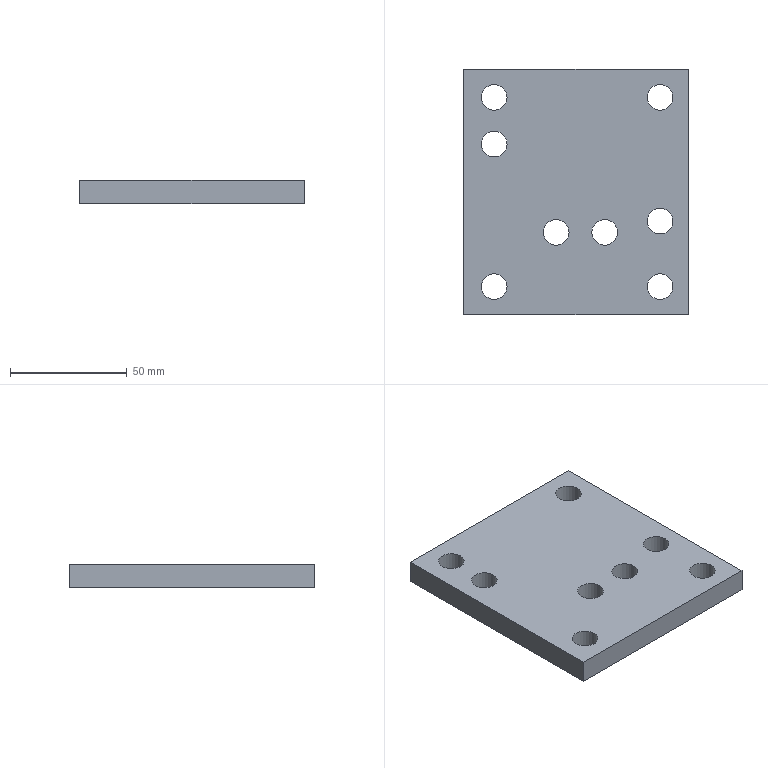Part | NX | features solid 2 | 1 solid | 14 faces | box 96 x 105 x 10 mm | volume 93197 mm3 | cylinder 8 | plane 6 | commonest cylinder face diameters 11 x8
STEP:
#1=CARTESIAN_POINT('',(298.719,-41.701,88.));
#2=VERTEX_POINT('',#1);
#3=CARTESIAN_POINT('',(298.719,63.299,88.));
#4=VERTEX_POINT('',#3);
#5=CARTESIAN_POINT('',(298.719,13.399,88.));
#6=DIRECTION('',(0.,1.,0.));
#7=VECTOR('',#6,1000.);
#8=LINE('',#5,#7);
#9=EDGE_CURVE('',#2,#4,#8,.T.);
#10=ORIENTED_EDGE('',*,*,#9,.T.);
#11=CARTESIAN_POINT('',(298.719,63.299,78.));
#12=VERTEX_POINT('',#11);
#13=CARTESIAN_POINT('',(298.719,63.299,78.));
#14=DIRECTION('',(0.,0.,-1.));
#15=VECTOR('',#14,1000.);
#16=LINE('',#13,#15);
#17=EDGE_CURVE('',#4,#12,#16,.T.);
#18=ORIENTED_EDGE('',*,*,#17,.T.);
#19=CARTESIAN_POINT('',(298.719,-41.701,78.));
#20=VERTEX_POINT('',#19);
#21=CARTESIAN_POINT('',(298.719,13.399,78.));
#22=DIRECTION('',(0.,1.,0.));
#23=VECTOR('',#22,1000.);
#24=LINE('',#21,#23);
#25=EDGE_CURVE('',#20,#12,#24,.T.);
#26=ORIENTED_EDGE('',*,*,#25,.F.);
#27=CARTESIAN_POINT('',(298.719,-41.701,78.));
#28=DIRECTION('',(0.,0.,-1.));
#29=VECTOR('',#28,1000.);
#30=LINE('',#27,#29);
#31=EDGE_CURVE('',#2,#20,#30,.T.);
#32=ORIENTED_EDGE('',*,*,#31,.F.);
#33=EDGE_LOOP('',(#10,#18,#26,#32));
#34=FACE_BOUND('',#33,.T.);
#35=CARTESIAN_POINT('',(298.719,13.399,78.));
#36=DIRECTION('',(1.,0.,0.));
#37=DIRECTION('',(0.,-1.,0.));
#38=AXIS2_PLACEMENT_3D('',#35,#36,#37);
#39=PLANE('',#38);
#40=ADVANCED_FACE('',(#34),#39,.F.);
#41=CARTESIAN_POINT('',(394.719,63.299,88.));
#42=VERTEX_POINT('',#41);
#43=CARTESIAN_POINT('',(394.719,63.299,78.));
#44=VERTEX_POINT('',#43);
#45=CARTESIAN_POINT('',(394.719,63.299,78.));
#46=DIRECTION('',(0.,0.,1.));
#47=VECTOR('',#46,1000.);
#48=LINE('',#45,#47);
#49=EDGE_CURVE('',#42,#44,#48,.F.);
#50=ORIENTED_EDGE('',*,*,#49,.T.);
#51=CARTESIAN_POINT('',(347.479,63.299,78.));
#52=DIRECTION('',(-1.,0.,0.));
#53=VECTOR('',#52,1000.);
#54=LINE('',#51,#53);
#55=EDGE_CURVE('',#12,#44,#54,.F.);
#56=ORIENTED_EDGE('',*,*,#55,.F.);
#57=ORIENTED_EDGE('',*,*,#17,.F.);
#58=CARTESIAN_POINT('',(188.,63.299,88.));
#59=DIRECTION('',(-1.,0.,0.));
#60=VECTOR('',#59,1000.);
#61=LINE('',#58,#60);
#62=EDGE_CURVE('',#4,#42,#61,.F.);
#63=ORIENTED_EDGE('',*,*,#62,.T.);
#64=EDGE_LOOP('',(#50,#56,#57,#63));
#65=FACE_BOUND('',#64,.T.);
#66=CARTESIAN_POINT('',(347.479,63.299,78.));
#67=DIRECTION('',(0.,-1.,0.));
#68=DIRECTION('',(-1.,0.,0.));
#69=AXIS2_PLACEMENT_3D('',#66,#67,#68);
#70=PLANE('',#69);
#71=ADVANCED_FACE('',(#65),#70,.F.);
#72=ORIENTED_EDGE('',*,*,#31,.T.);
#73=CARTESIAN_POINT('',(394.719,-41.701,78.));
#74=VERTEX_POINT('',#73);
#75=CARTESIAN_POINT('',(347.479,-41.701,78.));
#76=DIRECTION('',(1.,0.,0.));
#77=VECTOR('',#76,1000.);
#78=LINE('',#75,#77);
#79=EDGE_CURVE('',#74,#20,#78,.F.);
#80=ORIENTED_EDGE('',*,*,#79,.F.);
#81=CARTESIAN_POINT('',(394.719,-41.701,88.));
#82=VERTEX_POINT('',#81);
#83=CARTESIAN_POINT('',(394.719,-41.701,78.));
#84=DIRECTION('',(0.,0.,1.));
#85=VECTOR('',#84,1000.);
#86=LINE('',#83,#85);
#87=EDGE_CURVE('',#82,#74,#86,.F.);
#88=ORIENTED_EDGE('',*,*,#87,.F.);
#89=CARTESIAN_POINT('',(188.,-41.701,88.));
#90=DIRECTION('',(-1.,0.,0.));
#91=VECTOR('',#90,1000.);
#92=LINE('',#89,#91);
#93=EDGE_CURVE('',#82,#2,#92,.T.);
#94=ORIENTED_EDGE('',*,*,#93,.T.);
#95=EDGE_LOOP('',(#72,#80,#88,#94));
#96=FACE_BOUND('',#95,.T.);
#97=CARTESIAN_POINT('',(347.479,-41.701,78.));
#98=DIRECTION('',(0.,1.,0.));
#99=DIRECTION('',(1.,0.,0.));
#100=AXIS2_PLACEMENT_3D('',#97,#98,#99);
#101=PLANE('',#100);
#102=ADVANCED_FACE('',(#96),#101,.F.);
#103=CARTESIAN_POINT('',(377.219,-1.701,78.));
#104=VERTEX_POINT('',#103);
#105=CARTESIAN_POINT('',(382.719,-1.701,78.));
#106=DIRECTION('',(0.,0.,-1.));
#107=DIRECTION('',(-1.,0.,0.));
#108=AXIS2_PLACEMENT_3D('',#105,#106,#107);
#109=CIRCLE('',#108,5.5);
#110=EDGE_CURVE('',#104,#104,#109,.F.);
#111=ORIENTED_EDGE('',*,*,#110,.F.);
#112=EDGE_LOOP('',(#111));
#113=FACE_BOUND('',#112,.T.);
#114=CARTESIAN_POINT('',(377.219,-1.701,88.));
#115=VERTEX_POINT('',#114);
#116=CARTESIAN_POINT('',(382.719,-1.701,88.));
#117=DIRECTION('',(0.,0.,-1.));
#118=DIRECTION('',(-1.,0.,0.));
#119=AXIS2_PLACEMENT_3D('',#116,#117,#118);
#120=CIRCLE('',#119,5.5);
#121=EDGE_CURVE('',#115,#115,#120,.F.);
#122=ORIENTED_EDGE('',*,*,#121,.T.);
#123=EDGE_LOOP('',(#122));
#124=FACE_BOUND('',#123,.T.);
#125=CARTESIAN_POINT('',(382.719,-1.701,78.));
#126=DIRECTION('',(0.,0.,-1.));
#127=DIRECTION('',(-1.,0.,0.));
#128=AXIS2_PLACEMENT_3D('',#125,#126,#127);
#129=CYLINDRICAL_SURFACE('',#128,5.5);
#130=ADVANCED_FACE('',(#113,#124),#129,.F.);
#131=CARTESIAN_POINT('',(306.219,31.299,78.));
#132=VERTEX_POINT('',#131);
#133=CARTESIAN_POINT('',(311.719,31.299,78.));
#134=DIRECTION('',(0.,0.,-1.));
#135=DIRECTION('',(-1.,0.,0.));
#136=AXIS2_PLACEMENT_3D('',#133,#134,#135);
#137=CIRCLE('',#136,5.5);
#138=EDGE_CURVE('',#132,#132,#137,.F.);
#139=ORIENTED_EDGE('',*,*,#138,.F.);
#140=EDGE_LOOP('',(#139));
#141=FACE_BOUND('',#140,.T.);
#142=CARTESIAN_POINT('',(306.219,31.299,88.));
#143=VERTEX_POINT('',#142);
#144=CARTESIAN_POINT('',(311.719,31.299,88.));
#145=DIRECTION('',(0.,0.,-1.));
#146=DIRECTION('',(-1.,0.,0.));
#147=AXIS2_PLACEMENT_3D('',#144,#145,#146);
#148=CIRCLE('',#147,5.5);
#149=EDGE_CURVE('',#143,#143,#148,.F.);
#150=ORIENTED_EDGE('',*,*,#149,.T.);
#151=EDGE_LOOP('',(#150));
#152=FACE_BOUND('',#151,.T.);
#153=CARTESIAN_POINT('',(311.719,31.299,78.));
#154=DIRECTION('',(0.,0.,-1.));
#155=DIRECTION('',(-1.,0.,0.));
#156=AXIS2_PLACEMENT_3D('',#153,#154,#155);
#157=CYLINDRICAL_SURFACE('',#156,5.5);
#158=ADVANCED_FACE('',(#141,#152),#157,.F.);
#159=CARTESIAN_POINT('',(306.219,51.299,78.));
#160=VERTEX_POINT('',#159);
#161=CARTESIAN_POINT('',(311.719,51.299,78.));
#162=DIRECTION('',(0.,0.,-1.));
#163=DIRECTION('',(-1.,0.,0.));
#164=AXIS2_PLACEMENT_3D('',#161,#162,#163);
#165=CIRCLE('',#164,5.5);
#166=EDGE_CURVE('',#160,#160,#165,.T.);
#167=ORIENTED_EDGE('',*,*,#166,.T.);
#168=EDGE_LOOP('',(#167));
#169=FACE_BOUND('',#168,.T.);
#170=CARTESIAN_POINT('',(306.219,51.299,88.));
#171=VERTEX_POINT('',#170);
#172=CARTESIAN_POINT('',(311.719,51.299,88.));
#173=DIRECTION('',(0.,0.,-1.));
#174=DIRECTION('',(-1.,0.,0.));
#175=AXIS2_PLACEMENT_3D('',#172,#173,#174);
#176=CIRCLE('',#175,5.5);
#177=EDGE_CURVE('',#171,#171,#176,.T.);
#178=ORIENTED_EDGE('',*,*,#177,.F.);
#179=EDGE_LOOP('',(#178));
#180=FACE_BOUND('',#179,.T.);
#181=CARTESIAN_POINT('',(311.719,51.299,78.));
#182=DIRECTION('',(0.,0.,-1.));
#183=DIRECTION('',(-1.,0.,0.));
#184=AXIS2_PLACEMENT_3D('',#181,#182,#183);
#185=CYLINDRICAL_SURFACE('',#184,5.5);
#186=ADVANCED_FACE('',(#169,#180),#185,.F.);
#187=CARTESIAN_POINT('',(377.219,51.299,78.));
#188=VERTEX_POINT('',#187);
#189=CARTESIAN_POINT('',(382.719,51.299,78.));
#190=DIRECTION('',(0.,0.,-1.));
#191=DIRECTION('',(-1.,0.,0.));
#192=AXIS2_PLACEMENT_3D('',#189,#190,#191);
#193=CIRCLE('',#192,5.5);
#194=EDGE_CURVE('',#188,#188,#193,.T.);
#195=ORIENTED_EDGE('',*,*,#194,.T.);
#196=EDGE_LOOP('',(#195));
#197=FACE_BOUND('',#196,.T.);
#198=CARTESIAN_POINT('',(377.219,51.299,88.));
#199=VERTEX_POINT('',#198);
#200=CARTESIAN_POINT('',(382.719,51.299,88.));
#201=DIRECTION('',(0.,0.,-1.));
#202=DIRECTION('',(-1.,0.,0.));
#203=AXIS2_PLACEMENT_3D('',#200,#201,#202);
#204=CIRCLE('',#203,5.5);
#205=EDGE_CURVE('',#199,#199,#204,.T.);
#206=ORIENTED_EDGE('',*,*,#205,.F.);
#207=EDGE_LOOP('',(#206));
#208=FACE_BOUND('',#207,.T.);
#209=CARTESIAN_POINT('',(382.719,51.299,78.));
#210=DIRECTION('',(0.,0.,-1.));
#211=DIRECTION('',(-1.,0.,0.));
#212=AXIS2_PLACEMENT_3D('',#209,#210,#211);
#213=CYLINDRICAL_SURFACE('',#212,5.5);
#214=ADVANCED_FACE('',(#197,#208),#213,.F.);
#215=CARTESIAN_POINT('',(377.219,-29.701,78.));
#216=VERTEX_POINT('',#215);
#217=CARTESIAN_POINT('',(382.719,-29.701,78.));
#218=DIRECTION('',(0.,0.,-1.));
#219=DIRECTION('',(-1.,0.,0.));
#220=AXIS2_PLACEMENT_3D('',#217,#218,#219);
#221=CIRCLE('',#220,5.5);
#222=EDGE_CURVE('',#216,#216,#221,.T.);
#223=ORIENTED_EDGE('',*,*,#222,.T.);
#224=EDGE_LOOP('',(#223));
#225=FACE_BOUND('',#224,.T.);
#226=CARTESIAN_POINT('',(377.219,-29.701,88.));
#227=VERTEX_POINT('',#226);
#228=CARTESIAN_POINT('',(382.719,-29.701,88.));
#229=DIRECTION('',(0.,0.,-1.));
#230=DIRECTION('',(-1.,0.,0.));
#231=AXIS2_PLACEMENT_3D('',#228,#229,#230);
#232=CIRCLE('',#231,5.5);
#233=EDGE_CURVE('',#227,#227,#232,.T.);
#234=ORIENTED_EDGE('',*,*,#233,.F.);
#235=EDGE_LOOP('',(#234));
#236=FACE_BOUND('',#235,.T.);
#237=CARTESIAN_POINT('',(382.719,-29.701,78.));
#238=DIRECTION('',(0.,0.,-1.));
#239=DIRECTION('',(-1.,0.,0.));
#240=AXIS2_PLACEMENT_3D('',#237,#238,#239);
#241=CYLINDRICAL_SURFACE('',#240,5.5);
#242=ADVANCED_FACE('',(#225,#236),#241,.F.);
#243=CARTESIAN_POINT('',(306.219,-29.701,78.));
#244=VERTEX_POINT('',#243);
#245=CARTESIAN_POINT('',(311.719,-29.701,78.));
#246=DIRECTION('',(0.,0.,-1.));
#247=DIRECTION('',(-1.,0.,0.));
#248=AXIS2_PLACEMENT_3D('',#245,#246,#247);
#249=CIRCLE('',#248,5.5);
#250=EDGE_CURVE('',#244,#244,#249,.F.);
#251=ORIENTED_EDGE('',*,*,#250,.F.);
#252=EDGE_LOOP('',(#251));
#253=FACE_BOUND('',#252,.T.);
#254=CARTESIAN_POINT('',(306.219,-29.701,88.));
#255=VERTEX_POINT('',#254);
#256=CARTESIAN_POINT('',(311.719,-29.701,88.));
#257=DIRECTION('',(0.,0.,-1.));
#258=DIRECTION('',(-1.,0.,0.));
#259=AXIS2_PLACEMENT_3D('',#256,#257,#258);
#260=CIRCLE('',#259,5.5);
#261=EDGE_CURVE('',#255,#255,#260,.F.);
#262=ORIENTED_EDGE('',*,*,#261,.T.);
#263=EDGE_LOOP('',(#262));
#264=FACE_BOUND('',#263,.T.);
#265=CARTESIAN_POINT('',(311.719,-29.701,78.));
#266=DIRECTION('',(0.,0.,-1.));
#267=DIRECTION('',(-1.,0.,0.));
#268=AXIS2_PLACEMENT_3D('',#265,#266,#267);
#269=CYLINDRICAL_SURFACE('',#268,5.5);
#270=ADVANCED_FACE('',(#253,#264),#269,.F.);
#271=CARTESIAN_POINT('',(394.719,0.,88.));
#272=DIRECTION('',(0.,1.,0.));
#273=VECTOR('',#272,1000.);
#274=LINE('',#271,#273);
#275=EDGE_CURVE('',#42,#82,#274,.F.);
#276=ORIENTED_EDGE('',*,*,#275,.T.);
#277=ORIENTED_EDGE('',*,*,#87,.T.);
#278=CARTESIAN_POINT('',(394.719,13.399,78.));
#279=DIRECTION('',(0.,1.,0.));
#280=VECTOR('',#279,1000.);
#281=LINE('',#278,#280);
#282=EDGE_CURVE('',#44,#74,#281,.F.);
#283=ORIENTED_EDGE('',*,*,#282,.F.);
#284=ORIENTED_EDGE('',*,*,#49,.F.);
#285=EDGE_LOOP('',(#276,#277,#283,#284));
#286=FACE_BOUND('',#285,.T.);
#287=CARTESIAN_POINT('',(394.719,13.399,78.));
#288=DIRECTION('',(-1.,0.,0.));
#289=DIRECTION('',(0.,1.,0.));
#290=AXIS2_PLACEMENT_3D('',#287,#288,#289);
#291=PLANE('',#290);
#292=ADVANCED_FACE('',(#286),#291,.F.);
#293=CARTESIAN_POINT('',(353.471,-6.5,78.));
#294=VERTEX_POINT('',#293);
#295=CARTESIAN_POINT('',(358.971,-6.5,78.));
#296=DIRECTION('',(-0.000000369,-0.000000231,-1.));
#297=DIRECTION('',(-1.,0.,0.000000369));
#298=AXIS2_PLACEMENT_3D('',#295,#296,#297);
#299=CIRCLE('',#298,5.5);
#300=EDGE_CURVE('',#294,#294,#299,.T.);
#301=ORIENTED_EDGE('',*,*,#300,.T.);
#302=EDGE_LOOP('',(#301));
#303=FACE_BOUND('',#302,.T.);
#304=CARTESIAN_POINT('',(353.471,-6.5,88.));
#305=VERTEX_POINT('',#304);
#306=CARTESIAN_POINT('',(358.971,-6.5,88.));
#307=DIRECTION('',(-0.000000369,-0.000000231,-1.));
#308=DIRECTION('',(-1.,0.,0.000000369));
#309=AXIS2_PLACEMENT_3D('',#306,#307,#308);
#310=CIRCLE('',#309,5.5);
#311=EDGE_CURVE('',#305,#305,#310,.T.);
#312=ORIENTED_EDGE('',*,*,#311,.F.);
#313=EDGE_LOOP('',(#312));
#314=FACE_BOUND('',#313,.T.);
#315=CARTESIAN_POINT('',(358.971,-6.5,78.));
#316=DIRECTION('',(-0.000000369,-0.000000231,-1.));
#317=DIRECTION('',(-1.,0.,0.000000369));
#318=AXIS2_PLACEMENT_3D('',#315,#316,#317);
#319=CYLINDRICAL_SURFACE('',#318,5.5);
#320=ADVANCED_FACE('',(#303,#314),#319,.F.);
#321=CARTESIAN_POINT('',(332.763,-6.5,78.));
#322=VERTEX_POINT('',#321);
#323=CARTESIAN_POINT('',(338.263,-6.5,78.));
#324=DIRECTION('',(-0.000000369,-0.000000231,-1.));
#325=DIRECTION('',(-1.,0.,0.000000369));
#326=AXIS2_PLACEMENT_3D('',#323,#324,#325);
#327=CIRCLE('',#326,5.5);
#328=EDGE_CURVE('',#322,#322,#327,.F.);
#329=ORIENTED_EDGE('',*,*,#328,.F.);
#330=EDGE_LOOP('',(#329));
#331=FACE_BOUND('',#330,.T.);
#332=CARTESIAN_POINT('',(332.763,-6.5,88.));
#333=VERTEX_POINT('',#332);
#334=CARTESIAN_POINT('',(338.263,-6.5,88.));
#335=DIRECTION('',(-0.000000369,-0.000000231,-1.));
#336=DIRECTION('',(-1.,0.,0.000000369));
#337=AXIS2_PLACEMENT_3D('',#334,#335,#336);
#338=CIRCLE('',#337,5.5);
#339=EDGE_CURVE('',#333,#333,#338,.F.);
#340=ORIENTED_EDGE('',*,*,#339,.T.);
#341=EDGE_LOOP('',(#340));
#342=FACE_BOUND('',#341,.T.);
#343=CARTESIAN_POINT('',(338.263,-6.5,78.));
#344=DIRECTION('',(-0.000000369,-0.000000231,-1.));
#345=DIRECTION('',(-1.,0.,0.000000369));
#346=AXIS2_PLACEMENT_3D('',#343,#344,#345);
#347=CYLINDRICAL_SURFACE('',#346,5.5);
#348=ADVANCED_FACE('',(#331,#342),#347,.F.);
#349=ORIENTED_EDGE('',*,*,#25,.T.);
#350=ORIENTED_EDGE('',*,*,#55,.T.);
#351=ORIENTED_EDGE('',*,*,#282,.T.);
#352=ORIENTED_EDGE('',*,*,#79,.T.);
#353=EDGE_LOOP('',(#349,#350,#351,#352));
#354=FACE_BOUND('',#353,.T.);
#355=ORIENTED_EDGE('',*,*,#300,.F.);
#356=EDGE_LOOP('',(#355));
#357=FACE_BOUND('',#356,.T.);
#358=ORIENTED_EDGE('',*,*,#328,.T.);
#359=EDGE_LOOP('',(#358));
#360=FACE_BOUND('',#359,.T.);
#361=ORIENTED_EDGE('',*,*,#110,.T.);
#362=EDGE_LOOP('',(#361));
#363=FACE_BOUND('',#362,.T.);
#364=ORIENTED_EDGE('',*,*,#138,.T.);
#365=EDGE_LOOP('',(#364));
#366=FACE_BOUND('',#365,.T.);
#367=ORIENTED_EDGE('',*,*,#166,.F.);
#368=EDGE_LOOP('',(#367));
#369=FACE_BOUND('',#368,.T.);
#370=ORIENTED_EDGE('',*,*,#194,.F.);
#371=EDGE_LOOP('',(#370));
#372=FACE_BOUND('',#371,.T.);
#373=ORIENTED_EDGE('',*,*,#222,.F.);
#374=EDGE_LOOP('',(#373));
#375=FACE_BOUND('',#374,.T.);
#376=ORIENTED_EDGE('',*,*,#250,.T.);
#377=EDGE_LOOP('',(#376));
#378=FACE_BOUND('',#377,.T.);
#379=CARTESIAN_POINT('',(188.,0.,78.));
#380=DIRECTION('',(0.,0.,-1.));
#381=DIRECTION('',(-1.,0.,0.));
#382=AXIS2_PLACEMENT_3D('',#379,#380,#381);
#383=PLANE('',#382);
#384=ADVANCED_FACE('',(#354,#357,#360,#363,#366,#369,#372,#375,#378),#383,.T.);
#385=ORIENTED_EDGE('',*,*,#311,.T.);
#386=EDGE_LOOP('',(#385));
#387=FACE_BOUND('',#386,.T.);
#388=ORIENTED_EDGE('',*,*,#339,.F.);
#389=EDGE_LOOP('',(#388));
#390=FACE_BOUND('',#389,.T.);
#391=ORIENTED_EDGE('',*,*,#121,.F.);
#392=EDGE_LOOP('',(#391));
#393=FACE_BOUND('',#392,.T.);
#394=ORIENTED_EDGE('',*,*,#149,.F.);
#395=EDGE_LOOP('',(#394));
#396=FACE_BOUND('',#395,.T.);
#397=ORIENTED_EDGE('',*,*,#177,.T.);
#398=EDGE_LOOP('',(#397));
#399=FACE_BOUND('',#398,.T.);
#400=ORIENTED_EDGE('',*,*,#205,.T.);
#401=EDGE_LOOP('',(#400));
#402=FACE_BOUND('',#401,.T.);
#403=ORIENTED_EDGE('',*,*,#233,.T.);
#404=EDGE_LOOP('',(#403));
#405=FACE_BOUND('',#404,.T.);
#406=ORIENTED_EDGE('',*,*,#261,.F.);
#407=EDGE_LOOP('',(#406));
#408=FACE_BOUND('',#407,.T.);
#409=ORIENTED_EDGE('',*,*,#62,.F.);
#410=ORIENTED_EDGE('',*,*,#9,.F.);
#411=ORIENTED_EDGE('',*,*,#93,.F.);
#412=ORIENTED_EDGE('',*,*,#275,.F.);
#413=EDGE_LOOP('',(#409,#410,#411,#412));
#414=FACE_BOUND('',#413,.T.);
#415=CARTESIAN_POINT('',(188.,0.,88.));
#416=DIRECTION('',(0.,0.,-1.));
#417=DIRECTION('',(-1.,0.,0.));
#418=AXIS2_PLACEMENT_3D('',#415,#416,#417);
#419=PLANE('',#418);
#420=ADVANCED_FACE('',(#387,#390,#393,#396,#399,#402,#405,#408,#414),#419,.F.);
#421=CLOSED_SHELL('',(#40,#71,#102,#130,#158,#186,#214,#242,#270,#292,#320,#348,#384,#420));
#422=MANIFOLD_SOLID_BREP('',#421);
#423=(LENGTH_UNIT()NAMED_UNIT(*)SI_UNIT(.MILLI.,.METRE.));
#424=UNCERTAINTY_MEASURE_WITH_UNIT(LENGTH_MEASURE(0.00001),#423,'','');
#425=(NAMED_UNIT(*)PLANE_ANGLE_UNIT()SI_UNIT($,.RADIAN.));
#426=(NAMED_UNIT(*)SI_UNIT($,.STERADIAN.)SOLID_ANGLE_UNIT());
#427=(GEOMETRIC_REPRESENTATION_CONTEXT(3)GLOBAL_UNCERTAINTY_ASSIGNED_CONTEXT((#424))GLOBAL_UNIT_ASSIGNED_CONTEXT((#423,#425,#426))REPRESENTATION_CONTEXT('',''));
#428=ADVANCED_BREP_SHAPE_REPRESENTATION('',(#422),#427);